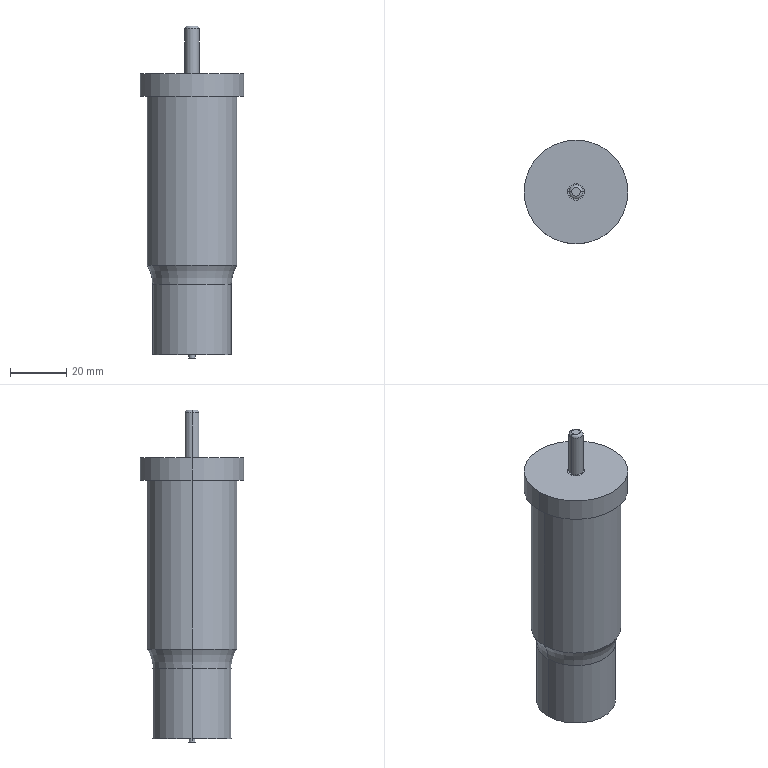Part | STEP file | 1_id3518_x_t | 1 solid | 22 faces | box 37 x 37 x 118.2 mm | volume 77419 mm3 | cylinder 12 | plane 6 | torus 4 | commonest cylinder face diameters 2.26 x2 5 x2 6 x2 28.07 x2 32 x2 37 x2
STEP:
#1=CARTESIAN_POINT('',(3253.867,-204.288,84.5));
#2=VERTEX_POINT('',#1);
#3=CARTESIAN_POINT('',(3253.867,-204.288,92.5));
#4=VERTEX_POINT('',#3);
#5=CARTESIAN_POINT('',(3253.867,-204.288,88.5));
#6=DIRECTION('',(0.,0.,1.));
#7=VECTOR('',#6,1.);
#8=LINE('',#5,#7);
#9=EDGE_CURVE('',#2,#4,#8,.T.);
#10=ORIENTED_EDGE('',*,*,#9,.F.);
#11=CARTESIAN_POINT('',(3216.867,-204.288,84.5));
#12=VERTEX_POINT('',#11);
#13=CARTESIAN_POINT('',(3235.367,-204.288,84.5));
#14=DIRECTION('',(0.,0.,1.));
#15=DIRECTION('',(1.,0.,0.));
#16=AXIS2_PLACEMENT_3D('',#13,#14,#15);
#17=CIRCLE('',#16,18.5);
#18=EDGE_CURVE('',#2,#12,#17,.T.);
#19=ORIENTED_EDGE('',*,*,#18,.T.);
#20=CARTESIAN_POINT('',(3216.867,-204.288,92.5));
#21=VERTEX_POINT('',#20);
#22=CARTESIAN_POINT('',(3216.867,-204.288,88.5));
#23=DIRECTION('',(0.,0.,-1.));
#24=VECTOR('',#23,1.);
#25=LINE('',#22,#24);
#26=EDGE_CURVE('',#21,#12,#25,.T.);
#27=ORIENTED_EDGE('',*,*,#26,.F.);
#28=CARTESIAN_POINT('',(3235.367,-204.288,92.5));
#29=DIRECTION('',(0.,0.,1.));
#30=DIRECTION('',(1.,0.,0.));
#31=AXIS2_PLACEMENT_3D('',#28,#29,#30);
#32=CIRCLE('',#31,18.5);
#33=EDGE_CURVE('',#4,#21,#32,.T.);
#34=ORIENTED_EDGE('',*,*,#33,.F.);
#35=EDGE_LOOP('',(#10,#19,#27,#34));
#36=FACE_OUTER_BOUND('',#35,.T.);
#37=CARTESIAN_POINT('',(3235.367,-204.288,88.5));
#38=DIRECTION('',(0.,0.,-1.));
#39=DIRECTION('',(-1.,0.,0.));
#40=AXIS2_PLACEMENT_3D('',#37,#38,#39);
#41=CYLINDRICAL_SURFACE('',#40,18.5);
#42=ADVANCED_FACE('',(#36),#41,.T.);
#43=CARTESIAN_POINT('',(3251.367,-204.288,24.372));
#44=VERTEX_POINT('',#43);
#45=CARTESIAN_POINT('',(3251.367,-204.288,84.5));
#46=VERTEX_POINT('',#45);
#47=CARTESIAN_POINT('',(3251.367,-204.288,38.5));
#48=DIRECTION('',(0.,0.,1.));
#49=VECTOR('',#48,1.);
#50=LINE('',#47,#49);
#51=EDGE_CURVE('',#44,#46,#50,.T.);
#52=ORIENTED_EDGE('',*,*,#51,.F.);
#53=CARTESIAN_POINT('',(3219.367,-204.288,24.372));
#54=VERTEX_POINT('',#53);
#55=CARTESIAN_POINT('',(3235.367,-204.288,24.372));
#56=DIRECTION('',(0.,0.,1.));
#57=DIRECTION('',(1.,0.,0.));
#58=AXIS2_PLACEMENT_3D('',#55,#56,#57);
#59=CIRCLE('',#58,16.);
#60=EDGE_CURVE('',#44,#54,#59,.T.);
#61=ORIENTED_EDGE('',*,*,#60,.T.);
#62=CARTESIAN_POINT('',(3219.367,-204.288,84.5));
#63=VERTEX_POINT('',#62);
#64=CARTESIAN_POINT('',(3219.367,-204.288,38.5));
#65=DIRECTION('',(0.,0.,-1.));
#66=VECTOR('',#65,1.);
#67=LINE('',#64,#66);
#68=EDGE_CURVE('',#63,#54,#67,.T.);
#69=ORIENTED_EDGE('',*,*,#68,.F.);
#70=CARTESIAN_POINT('',(3235.367,-204.288,84.5));
#71=DIRECTION('',(0.,0.,1.));
#72=DIRECTION('',(1.,0.,0.));
#73=AXIS2_PLACEMENT_3D('',#70,#71,#72);
#74=CIRCLE('',#73,16.);
#75=EDGE_CURVE('',#46,#63,#74,.T.);
#76=ORIENTED_EDGE('',*,*,#75,.F.);
#77=EDGE_LOOP('',(#52,#61,#69,#76));
#78=FACE_OUTER_BOUND('',#77,.T.);
#79=CARTESIAN_POINT('',(3235.367,-204.288,38.5));
#80=DIRECTION('',(0.,0.,-1.));
#81=DIRECTION('',(-1.,0.,0.));
#82=AXIS2_PLACEMENT_3D('',#79,#80,#81);
#83=CYLINDRICAL_SURFACE('',#82,16.);
#84=ADVANCED_FACE('',(#78),#83,.T.);
#85=CARTESIAN_POINT('',(3249.402,-204.288,17.5));
#86=VERTEX_POINT('',#85);
#87=CARTESIAN_POINT('',(3249.402,-204.288,-7.5));
#88=VERTEX_POINT('',#87);
#89=CARTESIAN_POINT('',(3249.402,-204.288,5.));
#90=DIRECTION('',(0.,0.,-1.));
#91=VECTOR('',#90,1.);
#92=LINE('',#89,#91);
#93=EDGE_CURVE('',#86,#88,#92,.T.);
#94=ORIENTED_EDGE('',*,*,#93,.F.);
#95=CARTESIAN_POINT('',(3221.332,-204.288,17.5));
#96=VERTEX_POINT('',#95);
#97=CARTESIAN_POINT('',(3235.367,-204.288,17.5));
#98=DIRECTION('',(0.,0.,1.));
#99=DIRECTION('',(1.,0.,0.));
#100=AXIS2_PLACEMENT_3D('',#97,#98,#99);
#101=CIRCLE('',#100,14.035);
#102=EDGE_CURVE('',#96,#86,#101,.T.);
#103=ORIENTED_EDGE('',*,*,#102,.F.);
#104=CARTESIAN_POINT('',(3221.332,-204.288,-7.5));
#105=VERTEX_POINT('',#104);
#106=CARTESIAN_POINT('',(3221.332,-204.288,5.));
#107=DIRECTION('',(0.,0.,1.));
#108=VECTOR('',#107,1.);
#109=LINE('',#106,#108);
#110=EDGE_CURVE('',#105,#96,#109,.T.);
#111=ORIENTED_EDGE('',*,*,#110,.F.);
#112=CARTESIAN_POINT('',(3235.367,-204.288,-7.5));
#113=DIRECTION('',(0.,0.,-1.));
#114=DIRECTION('',(1.,0.,0.));
#115=AXIS2_PLACEMENT_3D('',#112,#113,#114);
#116=CIRCLE('',#115,14.035);
#117=EDGE_CURVE('',#88,#105,#116,.T.);
#118=ORIENTED_EDGE('',*,*,#117,.F.);
#119=EDGE_LOOP('',(#94,#103,#111,#118));
#120=FACE_OUTER_BOUND('',#119,.T.);
#121=CARTESIAN_POINT('',(3235.367,-204.288,5.));
#122=DIRECTION('',(0.,0.,-1.));
#123=DIRECTION('',(-1.,0.,0.));
#124=AXIS2_PLACEMENT_3D('',#121,#122,#123);
#125=CYLINDRICAL_SURFACE('',#124,14.035);
#126=ADVANCED_FACE('',(#120),#125,.T.);
#127=CARTESIAN_POINT('',(3208.332,-204.288,17.5));
#128=DIRECTION('',(0.,-1.,0.));
#129=DIRECTION('',(-1.,0.,0.));
#130=AXIS2_PLACEMENT_3D('',#127,#128,#129);
#131=CIRCLE('',#130,13.);
#132=EDGE_CURVE('',#96,#54,#131,.T.);
#133=ORIENTED_EDGE('',*,*,#132,.F.);
#134=ORIENTED_EDGE('',*,*,#102,.T.);
#135=CARTESIAN_POINT('',(3262.402,-204.288,17.5));
#136=DIRECTION('',(0.,-1.,0.));
#137=DIRECTION('',(1.,0.,0.));
#138=AXIS2_PLACEMENT_3D('',#135,#136,#137);
#139=CIRCLE('',#138,13.);
#140=EDGE_CURVE('',#44,#86,#139,.T.);
#141=ORIENTED_EDGE('',*,*,#140,.F.);
#142=CARTESIAN_POINT('',(3235.367,-204.288,24.372));
#143=DIRECTION('',(0.,0.,1.));
#144=DIRECTION('',(1.,0.,0.));
#145=AXIS2_PLACEMENT_3D('',#142,#143,#144);
#146=CIRCLE('',#145,16.);
#147=EDGE_CURVE('',#54,#44,#146,.T.);
#148=ORIENTED_EDGE('',*,*,#147,.F.);
#149=EDGE_LOOP('',(#133,#134,#141,#148));
#150=FACE_OUTER_BOUND('',#149,.T.);
#151=CARTESIAN_POINT('',(3235.367,-204.288,17.5));
#152=DIRECTION('',(0.,0.,1.));
#153=DIRECTION('',(1.,0.,0.));
#154=AXIS2_PLACEMENT_3D('',#151,#152,#153);
#155=TOROIDAL_SURFACE('',#154,27.035,13.);
#156=ADVANCED_FACE('',(#150),#155,.F.);
#157=CARTESIAN_POINT('',(3234.237,-204.288,-7.5));
#158=VERTEX_POINT('',#157);
#159=CARTESIAN_POINT('',(3234.237,-204.288,-8.7));
#160=VERTEX_POINT('',#159);
#161=CARTESIAN_POINT('',(3234.237,-204.288,-7.5));
#162=DIRECTION('',(0.,0.,-1.));
#163=VECTOR('',#162,1.);
#164=LINE('',#161,#163);
#165=EDGE_CURVE('',#158,#160,#164,.T.);
#166=ORIENTED_EDGE('',*,*,#165,.F.);
#167=CARTESIAN_POINT('',(3236.497,-204.288,-7.5));
#168=VERTEX_POINT('',#167);
#169=CARTESIAN_POINT('',(3235.367,-204.288,-7.5));
#170=DIRECTION('',(0.,0.,1.));
#171=DIRECTION('',(-1.,0.,0.));
#172=AXIS2_PLACEMENT_3D('',#169,#170,#171);
#173=CIRCLE('',#172,1.13);
#174=EDGE_CURVE('',#168,#158,#173,.T.);
#175=ORIENTED_EDGE('',*,*,#174,.F.);
#176=CARTESIAN_POINT('',(3236.497,-204.288,-8.7));
#177=VERTEX_POINT('',#176);
#178=CARTESIAN_POINT('',(3236.497,-204.288,-7.5));
#179=DIRECTION('',(0.,0.,1.));
#180=VECTOR('',#179,1.);
#181=LINE('',#178,#180);
#182=EDGE_CURVE('',#177,#168,#181,.T.);
#183=ORIENTED_EDGE('',*,*,#182,.F.);
#184=CARTESIAN_POINT('',(3235.367,-204.288,-8.7));
#185=DIRECTION('',(0.,0.,1.));
#186=DIRECTION('',(-1.,0.,0.));
#187=AXIS2_PLACEMENT_3D('',#184,#185,#186);
#188=CIRCLE('',#187,1.13);
#189=EDGE_CURVE('',#177,#160,#188,.T.);
#190=ORIENTED_EDGE('',*,*,#189,.T.);
#191=EDGE_LOOP('',(#166,#175,#183,#190));
#192=FACE_OUTER_BOUND('',#191,.T.);
#193=CARTESIAN_POINT('',(3235.367,-204.288,-7.5));
#194=DIRECTION('',(0.,0.,1.));
#195=DIRECTION('',(1.,0.,0.));
#196=AXIS2_PLACEMENT_3D('',#193,#194,#195);
#197=CYLINDRICAL_SURFACE('',#196,1.13);
#198=ADVANCED_FACE('',(#192),#197,.T.);
#199=CARTESIAN_POINT('',(3232.867,-204.288,108.5));
#200=VERTEX_POINT('',#199);
#201=CARTESIAN_POINT('',(3232.867,-204.288,92.6));
#202=VERTEX_POINT('',#201);
#203=CARTESIAN_POINT('',(3232.867,-204.288,100.55));
#204=DIRECTION('',(0.,0.,-1.));
#205=VECTOR('',#204,1.);
#206=LINE('',#203,#205);
#207=EDGE_CURVE('',#200,#202,#206,.T.);
#208=ORIENTED_EDGE('',*,*,#207,.F.);
#209=CARTESIAN_POINT('',(3237.867,-204.288,108.5));
#210=VERTEX_POINT('',#209);
#211=CARTESIAN_POINT('',(3235.367,-204.288,108.5));
#212=DIRECTION('',(0.,0.,-1.));
#213=DIRECTION('',(-1.,0.,0.));
#214=AXIS2_PLACEMENT_3D('',#211,#212,#213);
#215=CIRCLE('',#214,2.5);
#216=EDGE_CURVE('',#200,#210,#215,.T.);
#217=ORIENTED_EDGE('',*,*,#216,.T.);
#218=CARTESIAN_POINT('',(3237.867,-204.288,92.6));
#219=VERTEX_POINT('',#218);
#220=CARTESIAN_POINT('',(3237.867,-204.288,100.55));
#221=DIRECTION('',(0.,0.,1.));
#222=VECTOR('',#221,1.);
#223=LINE('',#220,#222);
#224=EDGE_CURVE('',#219,#210,#223,.T.);
#225=ORIENTED_EDGE('',*,*,#224,.F.);
#226=CARTESIAN_POINT('',(3235.367,-204.288,92.6));
#227=DIRECTION('',(0.,0.,-1.));
#228=DIRECTION('',(-1.,0.,0.));
#229=AXIS2_PLACEMENT_3D('',#226,#227,#228);
#230=CIRCLE('',#229,2.5);
#231=EDGE_CURVE('',#202,#219,#230,.T.);
#232=ORIENTED_EDGE('',*,*,#231,.F.);
#233=EDGE_LOOP('',(#208,#217,#225,#232));
#234=FACE_OUTER_BOUND('',#233,.T.);
#235=CARTESIAN_POINT('',(3235.367,-204.288,100.55));
#236=DIRECTION('',(0.,0.,1.));
#237=DIRECTION('',(1.,0.,0.));
#238=AXIS2_PLACEMENT_3D('',#235,#236,#237);
#239=CYLINDRICAL_SURFACE('',#238,2.5);
#240=ADVANCED_FACE('',(#234),#239,.T.);
#241=CARTESIAN_POINT('',(3236.867,-204.288,109.5));
#242=VERTEX_POINT('',#241);
#243=CARTESIAN_POINT('',(3236.867,-204.288,108.5));
#244=DIRECTION('',(0.,1.,0.));
#245=DIRECTION('',(1.,0.,0.));
#246=AXIS2_PLACEMENT_3D('',#243,#244,#245);
#247=CIRCLE('',#246,1.);
#248=EDGE_CURVE('',#242,#210,#247,.T.);
#249=ORIENTED_EDGE('',*,*,#248,.F.);
#250=CARTESIAN_POINT('',(3233.867,-204.288,109.5));
#251=VERTEX_POINT('',#250);
#252=CARTESIAN_POINT('',(3235.367,-204.288,109.5));
#253=DIRECTION('',(0.,0.,-1.));
#254=DIRECTION('',(-1.,0.,0.));
#255=AXIS2_PLACEMENT_3D('',#252,#253,#254);
#256=CIRCLE('',#255,1.5);
#257=EDGE_CURVE('',#242,#251,#256,.T.);
#258=ORIENTED_EDGE('',*,*,#257,.T.);
#259=CARTESIAN_POINT('',(3233.867,-204.288,108.5));
#260=DIRECTION('',(0.,1.,0.));
#261=DIRECTION('',(-1.,0.,0.));
#262=AXIS2_PLACEMENT_3D('',#259,#260,#261);
#263=CIRCLE('',#262,1.);
#264=EDGE_CURVE('',#200,#251,#263,.T.);
#265=ORIENTED_EDGE('',*,*,#264,.F.);
#266=CARTESIAN_POINT('',(3235.367,-204.288,108.5));
#267=DIRECTION('',(0.,0.,-1.));
#268=DIRECTION('',(-1.,0.,0.));
#269=AXIS2_PLACEMENT_3D('',#266,#267,#268);
#270=CIRCLE('',#269,2.5);
#271=EDGE_CURVE('',#210,#200,#270,.T.);
#272=ORIENTED_EDGE('',*,*,#271,.F.);
#273=EDGE_LOOP('',(#249,#258,#265,#272));
#274=FACE_OUTER_BOUND('',#273,.T.);
#275=CARTESIAN_POINT('',(3235.367,-204.288,108.5));
#276=DIRECTION('',(0.,0.,-1.));
#277=DIRECTION('',(-1.,0.,0.));
#278=AXIS2_PLACEMENT_3D('',#275,#276,#277);
#279=TOROIDAL_SURFACE('',#278,1.5,1.);
#280=ADVANCED_FACE('',(#274),#279,.T.);
#281=CARTESIAN_POINT('',(3232.367,-204.288,92.6));
#282=VERTEX_POINT('',#281);
#283=CARTESIAN_POINT('',(3232.367,-204.288,92.5));
#284=VERTEX_POINT('',#283);
#285=CARTESIAN_POINT('',(3232.367,-204.288,92.55));
#286=DIRECTION('',(0.,0.,-1.));
#287=VECTOR('',#286,1.);
#288=LINE('',#285,#287);
#289=EDGE_CURVE('',#282,#284,#288,.T.);
#290=ORIENTED_EDGE('',*,*,#289,.F.);
#291=CARTESIAN_POINT('',(3238.367,-204.288,92.6));
#292=VERTEX_POINT('',#291);
#293=CARTESIAN_POINT('',(3235.367,-204.288,92.6));
#294=DIRECTION('',(0.,0.,-1.));
#295=DIRECTION('',(-1.,0.,0.));
#296=AXIS2_PLACEMENT_3D('',#293,#294,#295);
#297=CIRCLE('',#296,3.);
#298=EDGE_CURVE('',#282,#292,#297,.T.);
#299=ORIENTED_EDGE('',*,*,#298,.T.);
#300=CARTESIAN_POINT('',(3238.367,-204.288,92.5));
#301=VERTEX_POINT('',#300);
#302=CARTESIAN_POINT('',(3238.367,-204.288,92.55));
#303=DIRECTION('',(0.,0.,1.));
#304=VECTOR('',#303,1.);
#305=LINE('',#302,#304);
#306=EDGE_CURVE('',#301,#292,#305,.T.);
#307=ORIENTED_EDGE('',*,*,#306,.F.);
#308=CARTESIAN_POINT('',(3235.367,-204.288,92.5));
#309=DIRECTION('',(0.,0.,-1.));
#310=DIRECTION('',(-1.,0.,0.));
#311=AXIS2_PLACEMENT_3D('',#308,#309,#310);
#312=CIRCLE('',#311,3.);
#313=EDGE_CURVE('',#284,#301,#312,.T.);
#314=ORIENTED_EDGE('',*,*,#313,.F.);
#315=EDGE_LOOP('',(#290,#299,#307,#314));
#316=FACE_OUTER_BOUND('',#315,.T.);
#317=CARTESIAN_POINT('',(3235.367,-204.288,87.05));
#318=DIRECTION('',(0.,0.,1.));
#319=DIRECTION('',(1.,0.,0.));
#320=AXIS2_PLACEMENT_3D('',#317,#318,#319);
#321=CYLINDRICAL_SURFACE('',#320,3.);
#322=ADVANCED_FACE('',(#316),#321,.T.);
#323=ORIENTED_EDGE('',*,*,#289,.T.);
#324=CARTESIAN_POINT('',(3235.367,-204.288,92.5));
#325=DIRECTION('',(0.,0.,-1.));
#326=DIRECTION('',(-1.,0.,0.));
#327=AXIS2_PLACEMENT_3D('',#324,#325,#326);
#328=CIRCLE('',#327,3.);
#329=EDGE_CURVE('',#301,#284,#328,.T.);
#330=ORIENTED_EDGE('',*,*,#329,.F.);
#331=ORIENTED_EDGE('',*,*,#306,.T.);
#332=CARTESIAN_POINT('',(3235.367,-204.288,92.6));
#333=DIRECTION('',(0.,0.,-1.));
#334=DIRECTION('',(-1.,0.,0.));
#335=AXIS2_PLACEMENT_3D('',#332,#333,#334);
#336=CIRCLE('',#335,3.);
#337=EDGE_CURVE('',#292,#282,#336,.T.);
#338=ORIENTED_EDGE('',*,*,#337,.T.);
#339=EDGE_LOOP('',(#323,#330,#331,#338));
#340=FACE_OUTER_BOUND('',#339,.T.);
#341=CARTESIAN_POINT('',(3235.367,-204.288,87.05));
#342=DIRECTION('',(0.,0.,1.));
#343=DIRECTION('',(1.,0.,0.));
#344=AXIS2_PLACEMENT_3D('',#341,#342,#343);
#345=CYLINDRICAL_SURFACE('',#344,3.);
#346=ADVANCED_FACE('',(#340),#345,.T.);
#347=CARTESIAN_POINT('',(3235.367,-204.288,109.5));
#348=DIRECTION('',(0.,0.,-1.));
#349=DIRECTION('',(-1.,0.,0.));
#350=AXIS2_PLACEMENT_3D('',#347,#348,#349);
#351=CIRCLE('',#350,1.5);
#352=EDGE_CURVE('',#251,#242,#351,.T.);
#353=ORIENTED_EDGE('',*,*,#352,.F.);
#354=ORIENTED_EDGE('',*,*,#257,.F.);
#355=EDGE_LOOP('',(#353,#354));
#356=FACE_OUTER_BOUND('',#355,.T.);
#357=CARTESIAN_POINT('',(3234.617,-204.288,109.5));
#358=DIRECTION('',(0.,0.,1.));
#359=DIRECTION('',(-1.,0.,0.));
#360=AXIS2_PLACEMENT_3D('',#357,#358,#359);
#361=PLANE('',#360);
#362=ADVANCED_FACE('',(#356),#361,.T.);
#363=ORIENTED_EDGE('',*,*,#248,.T.);
#364=ORIENTED_EDGE('',*,*,#216,.F.);
#365=ORIENTED_EDGE('',*,*,#264,.T.);
#366=ORIENTED_EDGE('',*,*,#352,.T.);
#367=EDGE_LOOP('',(#363,#364,#365,#366));
#368=FACE_OUTER_BOUND('',#367,.T.);
#369=CARTESIAN_POINT('',(3235.367,-204.288,108.5));
#370=DIRECTION('',(0.,0.,-1.));
#371=DIRECTION('',(-1.,0.,0.));
#372=AXIS2_PLACEMENT_3D('',#369,#370,#371);
#373=TOROIDAL_SURFACE('',#372,1.5,1.);
#374=ADVANCED_FACE('',(#368),#373,.T.);
#375=ORIENTED_EDGE('',*,*,#207,.T.);
#376=CARTESIAN_POINT('',(3235.367,-204.288,92.6));
#377=DIRECTION('',(0.,0.,-1.));
#378=DIRECTION('',(-1.,0.,0.));
#379=AXIS2_PLACEMENT_3D('',#376,#377,#378);
#380=CIRCLE('',#379,2.5);
#381=EDGE_CURVE('',#219,#202,#380,.T.);
#382=ORIENTED_EDGE('',*,*,#381,.F.);
#383=ORIENTED_EDGE('',*,*,#224,.T.);
#384=ORIENTED_EDGE('',*,*,#271,.T.);
#385=EDGE_LOOP('',(#375,#382,#383,#384));
#386=FACE_OUTER_BOUND('',#385,.T.);
#387=CARTESIAN_POINT('',(3235.367,-204.288,100.55));
#388=DIRECTION('',(0.,0.,1.));
#389=DIRECTION('',(1.,0.,0.));
#390=AXIS2_PLACEMENT_3D('',#387,#388,#389);
#391=CYLINDRICAL_SURFACE('',#390,2.5);
#392=ADVANCED_FACE('',(#386),#391,.T.);
#393=ORIENTED_EDGE('',*,*,#298,.F.);
#394=ORIENTED_EDGE('',*,*,#337,.F.);
#395=EDGE_LOOP('',(#393,#394));
#396=FACE_BOUND('',#395,.T.);
#397=ORIENTED_EDGE('',*,*,#231,.T.);
#398=ORIENTED_EDGE('',*,*,#381,.T.);
#399=EDGE_LOOP('',(#397,#398));
#400=FACE_BOUND('',#399,.T.);
#401=CARTESIAN_POINT('',(3232.617,-204.288,92.6));
#402=DIRECTION('',(0.,0.,1.));
#403=DIRECTION('',(-1.,0.,0.));
#404=AXIS2_PLACEMENT_3D('',#401,#402,#403);
#405=PLANE('',#404);
#406=ADVANCED_FACE('',(#396,#400),#405,.T.);
#407=ORIENTED_EDGE('',*,*,#165,.T.);
#408=CARTESIAN_POINT('',(3235.367,-204.288,-8.7));
#409=DIRECTION('',(0.,0.,1.));
#410=DIRECTION('',(-1.,0.,0.));
#411=AXIS2_PLACEMENT_3D('',#408,#409,#410);
#412=CIRCLE('',#411,1.13);
#413=EDGE_CURVE('',#160,#177,#412,.T.);
#414=ORIENTED_EDGE('',*,*,#413,.T.);
#415=ORIENTED_EDGE('',*,*,#182,.T.);
#416=CARTESIAN_POINT('',(3235.367,-204.288,-7.5));
#417=DIRECTION('',(0.,0.,1.));
#418=DIRECTION('',(-1.,0.,0.));
#419=AXIS2_PLACEMENT_3D('',#416,#417,#418);
#420=CIRCLE('',#419,1.13);
#421=EDGE_CURVE('',#158,#168,#420,.T.);
#422=ORIENTED_EDGE('',*,*,#421,.F.);
#423=EDGE_LOOP('',(#407,#414,#415,#422));
#424=FACE_OUTER_BOUND('',#423,.T.);
#425=CARTESIAN_POINT('',(3235.367,-204.288,-7.5));
#426=DIRECTION('',(0.,0.,1.));
#427=DIRECTION('',(1.,0.,0.));
#428=AXIS2_PLACEMENT_3D('',#425,#426,#427);
#429=CYLINDRICAL_SURFACE('',#428,1.13);
#430=ADVANCED_FACE('',(#424),#429,.T.);
#431=ORIENTED_EDGE('',*,*,#413,.F.);
#432=ORIENTED_EDGE('',*,*,#189,.F.);
#433=EDGE_LOOP('',(#431,#432));
#434=FACE_OUTER_BOUND('',#433,.T.);
#435=CARTESIAN_POINT('',(3235.367,-204.288,-8.7));
#436=DIRECTION('',(0.,0.,1.));
#437=DIRECTION('',(1.,0.,0.));
#438=AXIS2_PLACEMENT_3D('',#435,#436,#437);
#439=PLANE('',#438);
#440=ADVANCED_FACE('',(#434),#439,.F.);
#441=ORIENTED_EDGE('',*,*,#132,.T.);
#442=ORIENTED_EDGE('',*,*,#60,.F.);
#443=ORIENTED_EDGE('',*,*,#140,.T.);
#444=CARTESIAN_POINT('',(3235.367,-204.288,17.5));
#445=DIRECTION('',(0.,0.,1.));
#446=DIRECTION('',(1.,0.,0.));
#447=AXIS2_PLACEMENT_3D('',#444,#445,#446);
#448=CIRCLE('',#447,14.035);
#449=EDGE_CURVE('',#86,#96,#448,.T.);
#450=ORIENTED_EDGE('',*,*,#449,.T.);
#451=EDGE_LOOP('',(#441,#442,#443,#450));
#452=FACE_OUTER_BOUND('',#451,.T.);
#453=CARTESIAN_POINT('',(3235.367,-204.288,17.5));
#454=DIRECTION('',(0.,0.,1.));
#455=DIRECTION('',(1.,0.,0.));
#456=AXIS2_PLACEMENT_3D('',#453,#454,#455);
#457=TOROIDAL_SURFACE('',#456,27.035,13.);
#458=ADVANCED_FACE('',(#452),#457,.F.);
#459=ORIENTED_EDGE('',*,*,#93,.T.);
#460=CARTESIAN_POINT('',(3235.367,-204.288,-7.5));
#461=DIRECTION('',(0.,0.,-1.));
#462=DIRECTION('',(1.,0.,0.));
#463=AXIS2_PLACEMENT_3D('',#460,#461,#462);
#464=CIRCLE('',#463,14.035);
#465=EDGE_CURVE('',#105,#88,#464,.T.);
#466=ORIENTED_EDGE('',*,*,#465,.F.);
#467=ORIENTED_EDGE('',*,*,#110,.T.);
#468=ORIENTED_EDGE('',*,*,#449,.F.);
#469=EDGE_LOOP('',(#459,#466,#467,#468));
#470=FACE_OUTER_BOUND('',#469,.T.);
#471=CARTESIAN_POINT('',(3235.367,-204.288,5.));
#472=DIRECTION('',(0.,0.,-1.));
#473=DIRECTION('',(-1.,0.,0.));
#474=AXIS2_PLACEMENT_3D('',#471,#472,#473);
#475=CYLINDRICAL_SURFACE('',#474,14.035);
#476=ADVANCED_FACE('',(#470),#475,.T.);
#477=ORIENTED_EDGE('',*,*,#421,.T.);
#478=ORIENTED_EDGE('',*,*,#174,.T.);
#479=EDGE_LOOP('',(#477,#478));
#480=FACE_BOUND('',#479,.T.);
#481=ORIENTED_EDGE('',*,*,#117,.T.);
#482=ORIENTED_EDGE('',*,*,#465,.T.);
#483=EDGE_LOOP('',(#481,#482));
#484=FACE_BOUND('',#483,.T.);
#485=CARTESIAN_POINT('',(3243.367,-204.288,-7.5));
#486=DIRECTION('',(0.,0.,-1.));
#487=DIRECTION('',(1.,0.,0.));
#488=AXIS2_PLACEMENT_3D('',#485,#486,#487);
#489=PLANE('',#488);
#490=ADVANCED_FACE('',(#480,#484),#489,.T.);
#491=ORIENTED_EDGE('',*,*,#51,.T.);
#492=CARTESIAN_POINT('',(3235.367,-204.288,84.5));
#493=DIRECTION('',(0.,0.,1.));
#494=DIRECTION('',(1.,0.,0.));
#495=AXIS2_PLACEMENT_3D('',#492,#493,#494);
#496=CIRCLE('',#495,16.);
#497=EDGE_CURVE('',#63,#46,#496,.T.);
#498=ORIENTED_EDGE('',*,*,#497,.F.);
#499=ORIENTED_EDGE('',*,*,#68,.T.);
#500=ORIENTED_EDGE('',*,*,#147,.T.);
#501=EDGE_LOOP('',(#491,#498,#499,#500));
#502=FACE_OUTER_BOUND('',#501,.T.);
#503=CARTESIAN_POINT('',(3235.367,-204.288,38.5));
#504=DIRECTION('',(0.,0.,-1.));
#505=DIRECTION('',(-1.,0.,0.));
#506=AXIS2_PLACEMENT_3D('',#503,#504,#505);
#507=CYLINDRICAL_SURFACE('',#506,16.);
#508=ADVANCED_FACE('',(#502),#507,.T.);
#509=ORIENTED_EDGE('',*,*,#18,.F.);
#510=CARTESIAN_POINT('',(3235.367,-204.288,84.5));
#511=DIRECTION('',(0.,0.,1.));
#512=DIRECTION('',(1.,0.,0.));
#513=AXIS2_PLACEMENT_3D('',#510,#511,#512);
#514=CIRCLE('',#513,18.5);
#515=EDGE_CURVE('',#12,#2,#514,.T.);
#516=ORIENTED_EDGE('',*,*,#515,.F.);
#517=EDGE_LOOP('',(#509,#516));
#518=FACE_BOUND('',#517,.T.);
#519=ORIENTED_EDGE('',*,*,#75,.T.);
#520=ORIENTED_EDGE('',*,*,#497,.T.);
#521=EDGE_LOOP('',(#519,#520));
#522=FACE_BOUND('',#521,.T.);
#523=CARTESIAN_POINT('',(3252.617,-204.288,84.5));
#524=DIRECTION('',(0.,0.,-1.));
#525=DIRECTION('',(1.,0.,0.));
#526=AXIS2_PLACEMENT_3D('',#523,#524,#525);
#527=PLANE('',#526);
#528=ADVANCED_FACE('',(#518,#522),#527,.T.);
#529=ORIENTED_EDGE('',*,*,#9,.T.);
#530=CARTESIAN_POINT('',(3235.367,-204.288,92.5));
#531=DIRECTION('',(0.,0.,1.));
#532=DIRECTION('',(1.,0.,0.));
#533=AXIS2_PLACEMENT_3D('',#530,#531,#532);
#534=CIRCLE('',#533,18.5);
#535=EDGE_CURVE('',#21,#4,#534,.T.);
#536=ORIENTED_EDGE('',*,*,#535,.F.);
#537=ORIENTED_EDGE('',*,*,#26,.T.);
#538=ORIENTED_EDGE('',*,*,#515,.T.);
#539=EDGE_LOOP('',(#529,#536,#537,#538));
#540=FACE_OUTER_BOUND('',#539,.T.);
#541=CARTESIAN_POINT('',(3235.367,-204.288,88.5));
#542=DIRECTION('',(0.,0.,-1.));
#543=DIRECTION('',(-1.,0.,0.));
#544=AXIS2_PLACEMENT_3D('',#541,#542,#543);
#545=CYLINDRICAL_SURFACE('',#544,18.5);
#546=ADVANCED_FACE('',(#540),#545,.T.);
#547=ORIENTED_EDGE('',*,*,#329,.T.);
#548=ORIENTED_EDGE('',*,*,#313,.T.);
#549=EDGE_LOOP('',(#547,#548));
#550=FACE_BOUND('',#549,.T.);
#551=ORIENTED_EDGE('',*,*,#33,.T.);
#552=ORIENTED_EDGE('',*,*,#535,.T.);
#553=EDGE_LOOP('',(#551,#552));
#554=FACE_BOUND('',#553,.T.);
#555=CARTESIAN_POINT('',(3244.617,-204.288,92.5));
#556=DIRECTION('',(0.,0.,1.));
#557=DIRECTION('',(-1.,0.,0.));
#558=AXIS2_PLACEMENT_3D('',#555,#556,#557);
#559=PLANE('',#558);
#560=ADVANCED_FACE('',(#550,#554),#559,.T.);
#561=CLOSED_SHELL('',(#42,#84,#126,#156,#198,#240,#280,#322,#346,#362,#374,#392,#406,#430,#440,#458,#476,#490,#508,#528,#546,#560));
#562=MANIFOLD_SOLID_BREP('',#561);
#563=(LENGTH_UNIT()NAMED_UNIT(*)SI_UNIT(.MILLI.,.METRE.));
#564=UNCERTAINTY_MEASURE_WITH_UNIT(LENGTH_MEASURE(0.00002),#563,'','');
#565=(NAMED_UNIT(*)PLANE_ANGLE_UNIT()SI_UNIT($,.RADIAN.));
#566=PLANE_ANGLE_MEASURE_WITH_UNIT(PLANE_ANGLE_MEASURE(0.01745),#565);
#567=DIMENSIONAL_EXPONENTS(0.,0.,0.,0.,0.,0.,0.);
#568=(CONVERSION_BASED_UNIT('DEGREE',#566)NAMED_UNIT(#567)PLANE_ANGLE_UNIT());
#569=(NAMED_UNIT(*)SI_UNIT($,.STERADIAN.)SOLID_ANGLE_UNIT());
#570=(GEOMETRIC_REPRESENTATION_CONTEXT(3)GLOBAL_UNCERTAINTY_ASSIGNED_CONTEXT((#564))GLOBAL_UNIT_ASSIGNED_CONTEXT((#563,#568,#569))REPRESENTATION_CONTEXT('',''));
#571=ADVANCED_BREP_SHAPE_REPRESENTATION('',(#562),#570);